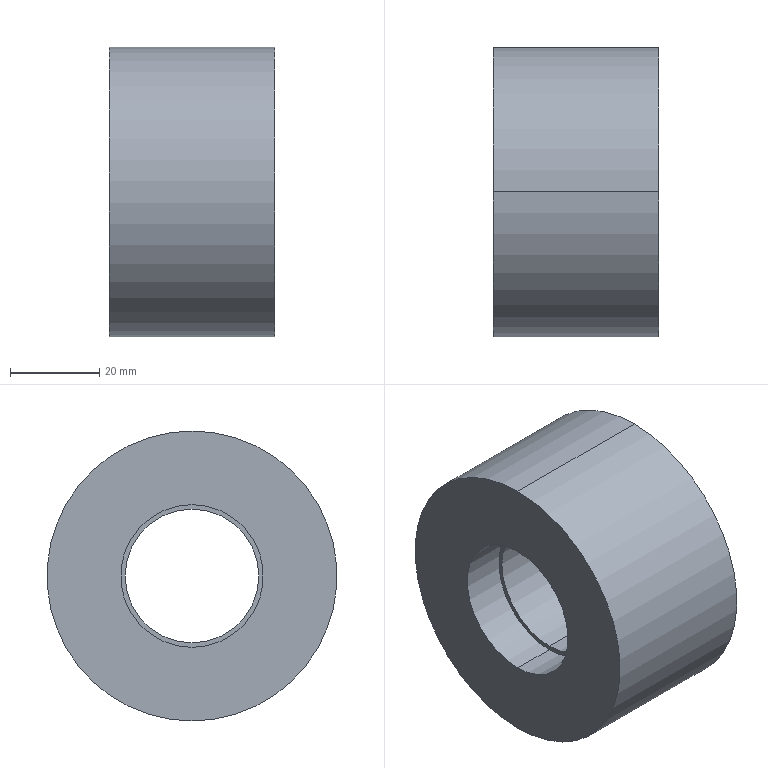Part | STEP file | 0245_Z_009_AFBD37-65_1 | 1 solid | 12 faces | box 37 x 65 x 65 mm | volume 94676 mm3 | cylinder 8 | plane 4 | commonest cylinder face diameters 32 x4 30 x2 65 x2
STEP:
#1=CARTESIAN_POINT('',(0.,0.,0.));
#2=DIRECTION('',(0.,0.,1.));
#3=DIRECTION('',(1.,0.,0.));
#4=AXIS2_PLACEMENT_3D('',#1,#2,#3);
#5=CARTESIAN_POINT('',(-18.5,0.,-32.5));
#6=VERTEX_POINT('',#5);
#7=CARTESIAN_POINT('',(-18.5,0.,32.5));
#8=VERTEX_POINT('',#7);
#9=CARTESIAN_POINT('',(-18.5,0.,0.));
#10=DIRECTION('',(1.,0.,0.));
#11=DIRECTION('',(0.,0.,-1.));
#12=AXIS2_PLACEMENT_3D('',#9,#10,#11);
#13=CIRCLE('',#12,32.5);
#14=CARTESIAN_POINT('',(0.,0.,0.));
#15=DIRECTION('',(1.,0.,0.));
#16=DIRECTION('',(0.,0.,-1.));
#17=AXIS2_PLACEMENT_3D('',#14,#15,#16);
#18=CYLINDRICAL_SURFACE('',#17,32.5);
#19=CARTESIAN_POINT('',(0.,-18.5));
#20=DIRECTION('',(1.,0.));
#21=VECTOR('',#20,1.);
#22=LINE('',#19,#21);
#23=(GEOMETRIC_REPRESENTATION_CONTEXT(2)PARAMETRIC_REPRESENTATION_CONTEXT()REPRESENTATION_CONTEXT('',''));
#24=DEFINITIONAL_REPRESENTATION('',(#22),#23);
#25=PCURVE('',#18,#24);
#26=CARTESIAN_POINT('',(-18.5,24.25,0.));
#27=DIRECTION('',(-1.,0.,0.));
#28=DIRECTION('',(0.,0.,1.));
#29=AXIS2_PLACEMENT_3D('',#26,#27,#28);
#30=PLANE('',#29);
#31=CARTESIAN_POINT('',(-32.5,-24.25));
#32=CARTESIAN_POINT('',(-32.5,32.042));
#33=CARTESIAN_POINT('',(16.25,3.896));
#34=CARTESIAN_POINT('',(65.,-24.25));
#35=CARTESIAN_POINT('',(16.25,-52.396));
#36=CARTESIAN_POINT('',(-32.5,-80.542));
#37=CARTESIAN_POINT('',(-32.5,-24.25));
#38=(BOUNDED_CURVE()B_SPLINE_CURVE(2,(#31,#32,#33,#34,#35,#36,#37),.UNSPECIFIED.,.T.,.F.)B_SPLINE_CURVE_WITH_KNOTS((1,2,2,2,2,1),(-2.094,0.,2.094,4.189,6.283,8.378),.UNSPECIFIED.)CURVE()GEOMETRIC_REPRESENTATION_ITEM()RATIONAL_B_SPLINE_CURVE((1.,0.5,1.,0.5,1.,0.5,1.))REPRESENTATION_ITEM(''));
#39=(GEOMETRIC_REPRESENTATION_CONTEXT(2)PARAMETRIC_REPRESENTATION_CONTEXT()REPRESENTATION_CONTEXT('',''));
#40=DEFINITIONAL_REPRESENTATION('',(#38),#39);
#41=PCURVE('',#30,#40);
#42=SURFACE_CURVE('',#13,(#25,#41),.PCURVE_S1.);
#43=EDGE_CURVE('',#6,#8,#42,.T.);
#44=ORIENTED_EDGE('',*,*,#43,.T.);
#45=CARTESIAN_POINT('',(18.5,0.,32.5));
#46=VERTEX_POINT('',#45);
#47=CARTESIAN_POINT('',(0.,0.,32.5));
#48=DIRECTION('',(1.,0.,0.));
#49=VECTOR('',#48,1.);
#50=LINE('',#47,#49);
#51=CARTESIAN_POINT('',(3.142,0.));
#52=DIRECTION('',(0.,1.));
#53=VECTOR('',#52,1.);
#54=LINE('',#51,#53);
#55=(GEOMETRIC_REPRESENTATION_CONTEXT(2)PARAMETRIC_REPRESENTATION_CONTEXT()REPRESENTATION_CONTEXT('',''));
#56=DEFINITIONAL_REPRESENTATION('',(#54),#55);
#57=PCURVE('',#18,#56);
#58=CARTESIAN_POINT('',(0.,0.,0.));
#59=DIRECTION('',(1.,0.,0.));
#60=DIRECTION('',(0.,0.,-1.));
#61=AXIS2_PLACEMENT_3D('',#58,#59,#60);
#62=CYLINDRICAL_SURFACE('',#61,32.5);
#63=CARTESIAN_POINT('',(3.142,0.));
#64=DIRECTION('',(0.,1.));
#65=VECTOR('',#64,1.);
#66=LINE('',#63,#65);
#67=(GEOMETRIC_REPRESENTATION_CONTEXT(2)PARAMETRIC_REPRESENTATION_CONTEXT()REPRESENTATION_CONTEXT('',''));
#68=DEFINITIONAL_REPRESENTATION('',(#66),#67);
#69=PCURVE('',#62,#68);
#70=SURFACE_CURVE('',#50,(#57,#69),.PCURVE_S1.);
#71=EDGE_CURVE('',#8,#46,#70,.T.);
#72=ORIENTED_EDGE('',*,*,#71,.T.);
#73=CARTESIAN_POINT('',(18.5,0.,-32.5));
#74=VERTEX_POINT('',#73);
#75=CARTESIAN_POINT('',(18.5,0.,0.));
#76=DIRECTION('',(-1.,0.,0.));
#77=DIRECTION('',(0.,0.,-1.));
#78=AXIS2_PLACEMENT_3D('',#75,#76,#77);
#79=CIRCLE('',#78,32.5);
#80=CARTESIAN_POINT('',(6.283,18.5));
#81=DIRECTION('',(-1.,0.));
#82=VECTOR('',#81,1.);
#83=LINE('',#80,#82);
#84=(GEOMETRIC_REPRESENTATION_CONTEXT(2)PARAMETRIC_REPRESENTATION_CONTEXT()REPRESENTATION_CONTEXT('',''));
#85=DEFINITIONAL_REPRESENTATION('',(#83),#84);
#86=PCURVE('',#18,#85);
#87=CARTESIAN_POINT('',(18.5,24.25,0.));
#88=DIRECTION('',(1.,0.,0.));
#89=DIRECTION('',(0.,0.,-1.));
#90=AXIS2_PLACEMENT_3D('',#87,#88,#89);
#91=PLANE('',#90);
#92=CARTESIAN_POINT('',(32.5,-24.25));
#93=CARTESIAN_POINT('',(32.5,-80.542));
#94=CARTESIAN_POINT('',(-16.25,-52.396));
#95=CARTESIAN_POINT('',(-65.,-24.25));
#96=CARTESIAN_POINT('',(-16.25,3.896));
#97=CARTESIAN_POINT('',(32.5,32.042));
#98=CARTESIAN_POINT('',(32.5,-24.25));
#99=(BOUNDED_CURVE()B_SPLINE_CURVE(2,(#92,#93,#94,#95,#96,#97,#98),.UNSPECIFIED.,.T.,.F.)B_SPLINE_CURVE_WITH_KNOTS((1,2,2,2,2,1),(-2.094,0.,2.094,4.189,6.283,8.378),.UNSPECIFIED.)CURVE()GEOMETRIC_REPRESENTATION_ITEM()RATIONAL_B_SPLINE_CURVE((1.,0.5,1.,0.5,1.,0.5,1.))REPRESENTATION_ITEM(''));
#100=(GEOMETRIC_REPRESENTATION_CONTEXT(2)PARAMETRIC_REPRESENTATION_CONTEXT()REPRESENTATION_CONTEXT('',''));
#101=DEFINITIONAL_REPRESENTATION('',(#99),#100);
#102=PCURVE('',#91,#101);
#103=SURFACE_CURVE('',#79,(#86,#102),.PCURVE_S1.);
#104=EDGE_CURVE('',#46,#74,#103,.T.);
#105=ORIENTED_EDGE('',*,*,#104,.T.);
#106=CARTESIAN_POINT('',(0.,0.,-32.5));
#107=DIRECTION('',(1.,0.,0.));
#108=VECTOR('',#107,1.);
#109=LINE('',#106,#108);
#110=CARTESIAN_POINT('',(0.,0.));
#111=DIRECTION('',(0.,1.));
#112=VECTOR('',#111,1.);
#113=LINE('',#110,#112);
#114=(GEOMETRIC_REPRESENTATION_CONTEXT(2)PARAMETRIC_REPRESENTATION_CONTEXT()REPRESENTATION_CONTEXT('',''));
#115=DEFINITIONAL_REPRESENTATION('',(#113),#114);
#116=PCURVE('',#18,#115);
#117=CARTESIAN_POINT('',(6.283,0.));
#118=DIRECTION('',(0.,1.));
#119=VECTOR('',#118,1.);
#120=LINE('',#117,#119);
#121=(GEOMETRIC_REPRESENTATION_CONTEXT(2)PARAMETRIC_REPRESENTATION_CONTEXT()REPRESENTATION_CONTEXT('',''));
#122=DEFINITIONAL_REPRESENTATION('',(#120),#121);
#123=PCURVE('',#62,#122);
#124=SURFACE_CURVE('',#109,(#116,#123),.PCURVE_S1.);
#125=EDGE_CURVE('',#6,#74,#124,.T.);
#126=ORIENTED_EDGE('',*,*,#125,.F.);
#127=EDGE_LOOP('',(#44,#72,#105,#126));
#128=FACE_BOUND('',#127,.T.);
#129=ADVANCED_FACE('',(#128),#18,.T.);
#130=CARTESIAN_POINT('',(-18.5,0.,-16.));
#131=VERTEX_POINT('',#130);
#132=CARTESIAN_POINT('',(-8.5,0.,-16.));
#133=VERTEX_POINT('',#132);
#134=CARTESIAN_POINT('',(-13.5,0.,-16.));
#135=DIRECTION('',(1.,0.,0.));
#136=VECTOR('',#135,1.);
#137=LINE('',#134,#136);
#138=CARTESIAN_POINT('',(-13.5,0.,0.));
#139=DIRECTION('',(1.,0.,0.));
#140=DIRECTION('',(0.,0.,-1.));
#141=AXIS2_PLACEMENT_3D('',#138,#139,#140);
#142=CYLINDRICAL_SURFACE('',#141,16.);
#143=CARTESIAN_POINT('',(6.283,0.));
#144=DIRECTION('',(0.,1.));
#145=VECTOR('',#144,1.);
#146=LINE('',#143,#145);
#147=(GEOMETRIC_REPRESENTATION_CONTEXT(2)PARAMETRIC_REPRESENTATION_CONTEXT()REPRESENTATION_CONTEXT('',''));
#148=DEFINITIONAL_REPRESENTATION('',(#146),#147);
#149=PCURVE('',#142,#148);
#150=CARTESIAN_POINT('',(-13.5,0.,0.));
#151=DIRECTION('',(1.,0.,0.));
#152=DIRECTION('',(0.,0.,-1.));
#153=AXIS2_PLACEMENT_3D('',#150,#151,#152);
#154=CYLINDRICAL_SURFACE('',#153,16.);
#155=CARTESIAN_POINT('',(0.,0.));
#156=DIRECTION('',(0.,1.));
#157=VECTOR('',#156,1.);
#158=LINE('',#155,#157);
#159=(GEOMETRIC_REPRESENTATION_CONTEXT(2)PARAMETRIC_REPRESENTATION_CONTEXT()REPRESENTATION_CONTEXT('',''));
#160=DEFINITIONAL_REPRESENTATION('',(#158),#159);
#161=PCURVE('',#154,#160);
#162=SURFACE_CURVE('',#137,(#149,#161),.PCURVE_S1.);
#163=EDGE_CURVE('',#131,#133,#162,.T.);
#164=ORIENTED_EDGE('',*,*,#163,.T.);
#165=CARTESIAN_POINT('',(-8.5,0.,16.));
#166=VERTEX_POINT('',#165);
#167=CARTESIAN_POINT('',(-8.5,0.,0.));
#168=DIRECTION('',(-1.,0.,0.));
#169=DIRECTION('',(0.,0.,-1.));
#170=AXIS2_PLACEMENT_3D('',#167,#168,#169);
#171=CIRCLE('',#170,16.);
#172=CARTESIAN_POINT('',(6.283,5.));
#173=DIRECTION('',(-1.,0.));
#174=VECTOR('',#173,1.);
#175=LINE('',#172,#174);
#176=(GEOMETRIC_REPRESENTATION_CONTEXT(2)PARAMETRIC_REPRESENTATION_CONTEXT()REPRESENTATION_CONTEXT('',''));
#177=DEFINITIONAL_REPRESENTATION('',(#175),#176);
#178=PCURVE('',#142,#177);
#179=CARTESIAN_POINT('',(-8.5,15.5,0.));
#180=DIRECTION('',(-1.,0.,0.));
#181=DIRECTION('',(0.,0.,1.));
#182=AXIS2_PLACEMENT_3D('',#179,#180,#181);
#183=PLANE('',#182);
#184=CARTESIAN_POINT('',(0.,-15.5));
#185=DIRECTION('',(-1.,0.));
#186=AXIS2_PLACEMENT_2D('',#184,#185);
#187=CIRCLE('',#186,16.);
#188=(GEOMETRIC_REPRESENTATION_CONTEXT(2)PARAMETRIC_REPRESENTATION_CONTEXT()REPRESENTATION_CONTEXT('',''));
#189=DEFINITIONAL_REPRESENTATION('',(#187),#188);
#190=PCURVE('',#183,#189);
#191=SURFACE_CURVE('',#171,(#178,#190),.PCURVE_S1.);
#192=EDGE_CURVE('',#133,#166,#191,.T.);
#193=ORIENTED_EDGE('',*,*,#192,.T.);
#194=CARTESIAN_POINT('',(-18.5,0.,16.));
#195=VERTEX_POINT('',#194);
#196=CARTESIAN_POINT('',(-13.5,0.,16.));
#197=DIRECTION('',(1.,0.,0.));
#198=VECTOR('',#197,1.);
#199=LINE('',#196,#198);
#200=CARTESIAN_POINT('',(3.142,0.));
#201=DIRECTION('',(0.,1.));
#202=VECTOR('',#201,1.);
#203=LINE('',#200,#202);
#204=(GEOMETRIC_REPRESENTATION_CONTEXT(2)PARAMETRIC_REPRESENTATION_CONTEXT()REPRESENTATION_CONTEXT('',''));
#205=DEFINITIONAL_REPRESENTATION('',(#203),#204);
#206=PCURVE('',#142,#205);
#207=CARTESIAN_POINT('',(3.142,0.));
#208=DIRECTION('',(0.,1.));
#209=VECTOR('',#208,1.);
#210=LINE('',#207,#209);
#211=(GEOMETRIC_REPRESENTATION_CONTEXT(2)PARAMETRIC_REPRESENTATION_CONTEXT()REPRESENTATION_CONTEXT('',''));
#212=DEFINITIONAL_REPRESENTATION('',(#210),#211);
#213=PCURVE('',#154,#212);
#214=SURFACE_CURVE('',#199,(#206,#213),.PCURVE_S1.);
#215=EDGE_CURVE('',#195,#166,#214,.T.);
#216=ORIENTED_EDGE('',*,*,#215,.F.);
#217=CARTESIAN_POINT('',(-18.5,0.,0.));
#218=DIRECTION('',(1.,0.,0.));
#219=DIRECTION('',(0.,0.,-1.));
#220=AXIS2_PLACEMENT_3D('',#217,#218,#219);
#221=CIRCLE('',#220,16.);
#222=CARTESIAN_POINT('',(0.,-5.));
#223=DIRECTION('',(1.,0.));
#224=VECTOR('',#223,1.);
#225=LINE('',#222,#224);
#226=(GEOMETRIC_REPRESENTATION_CONTEXT(2)PARAMETRIC_REPRESENTATION_CONTEXT()REPRESENTATION_CONTEXT('',''));
#227=DEFINITIONAL_REPRESENTATION('',(#225),#226);
#228=PCURVE('',#142,#227);
#229=CARTESIAN_POINT('',(-16.,-24.25));
#230=CARTESIAN_POINT('',(-16.,3.463));
#231=CARTESIAN_POINT('',(8.,-10.394));
#232=CARTESIAN_POINT('',(32.,-24.25));
#233=CARTESIAN_POINT('',(8.,-38.106));
#234=CARTESIAN_POINT('',(-16.,-51.963));
#235=CARTESIAN_POINT('',(-16.,-24.25));
#236=(BOUNDED_CURVE()B_SPLINE_CURVE(2,(#229,#230,#231,#232,#233,#234,#235),.UNSPECIFIED.,.T.,.F.)B_SPLINE_CURVE_WITH_KNOTS((1,2,2,2,2,1),(-2.094,0.,2.094,4.189,6.283,8.378),.UNSPECIFIED.)CURVE()GEOMETRIC_REPRESENTATION_ITEM()RATIONAL_B_SPLINE_CURVE((1.,0.5,1.,0.5,1.,0.5,1.))REPRESENTATION_ITEM(''));
#237=(GEOMETRIC_REPRESENTATION_CONTEXT(2)PARAMETRIC_REPRESENTATION_CONTEXT()REPRESENTATION_CONTEXT('',''));
#238=DEFINITIONAL_REPRESENTATION('',(#236),#237);
#239=PCURVE('',#30,#238);
#240=SURFACE_CURVE('',#221,(#228,#239),.PCURVE_S1.);
#241=EDGE_CURVE('',#195,#131,#240,.T.);
#242=ORIENTED_EDGE('',*,*,#241,.T.);
#243=EDGE_LOOP('',(#164,#193,#216,#242));
#244=FACE_BOUND('',#243,.F.);
#245=ADVANCED_FACE('',(#244),#142,.F.);
#246=CARTESIAN_POINT('',(8.5,0.,-16.));
#247=VERTEX_POINT('',#246);
#248=CARTESIAN_POINT('',(18.5,0.,-16.));
#249=VERTEX_POINT('',#248);
#250=CARTESIAN_POINT('',(13.5,0.,-16.));
#251=DIRECTION('',(1.,0.,0.));
#252=VECTOR('',#251,1.);
#253=LINE('',#250,#252);
#254=CARTESIAN_POINT('',(13.5,0.,0.));
#255=DIRECTION('',(1.,0.,0.));
#256=DIRECTION('',(0.,0.,-1.));
#257=AXIS2_PLACEMENT_3D('',#254,#255,#256);
#258=CYLINDRICAL_SURFACE('',#257,16.);
#259=CARTESIAN_POINT('',(6.283,0.));
#260=DIRECTION('',(0.,1.));
#261=VECTOR('',#260,1.);
#262=LINE('',#259,#261);
#263=(GEOMETRIC_REPRESENTATION_CONTEXT(2)PARAMETRIC_REPRESENTATION_CONTEXT()REPRESENTATION_CONTEXT('',''));
#264=DEFINITIONAL_REPRESENTATION('',(#262),#263);
#265=PCURVE('',#258,#264);
#266=CARTESIAN_POINT('',(13.5,0.,0.));
#267=DIRECTION('',(1.,0.,0.));
#268=DIRECTION('',(0.,0.,-1.));
#269=AXIS2_PLACEMENT_3D('',#266,#267,#268);
#270=CYLINDRICAL_SURFACE('',#269,16.);
#271=CARTESIAN_POINT('',(0.,0.));
#272=DIRECTION('',(0.,1.));
#273=VECTOR('',#272,1.);
#274=LINE('',#271,#273);
#275=(GEOMETRIC_REPRESENTATION_CONTEXT(2)PARAMETRIC_REPRESENTATION_CONTEXT()REPRESENTATION_CONTEXT('',''));
#276=DEFINITIONAL_REPRESENTATION('',(#274),#275);
#277=PCURVE('',#270,#276);
#278=SURFACE_CURVE('',#253,(#265,#277),.PCURVE_S1.);
#279=EDGE_CURVE('',#247,#249,#278,.T.);
#280=ORIENTED_EDGE('',*,*,#279,.T.);
#281=CARTESIAN_POINT('',(18.5,0.,16.));
#282=VERTEX_POINT('',#281);
#283=CARTESIAN_POINT('',(18.5,0.,0.));
#284=DIRECTION('',(-1.,0.,0.));
#285=DIRECTION('',(0.,0.,-1.));
#286=AXIS2_PLACEMENT_3D('',#283,#284,#285);
#287=CIRCLE('',#286,16.);
#288=CARTESIAN_POINT('',(6.283,5.));
#289=DIRECTION('',(-1.,0.));
#290=VECTOR('',#289,1.);
#291=LINE('',#288,#290);
#292=(GEOMETRIC_REPRESENTATION_CONTEXT(2)PARAMETRIC_REPRESENTATION_CONTEXT()REPRESENTATION_CONTEXT('',''));
#293=DEFINITIONAL_REPRESENTATION('',(#291),#292);
#294=PCURVE('',#258,#293);
#295=CARTESIAN_POINT('',(16.,-24.25));
#296=CARTESIAN_POINT('',(16.,-51.963));
#297=CARTESIAN_POINT('',(-8.,-38.106));
#298=CARTESIAN_POINT('',(-32.,-24.25));
#299=CARTESIAN_POINT('',(-8.,-10.394));
#300=CARTESIAN_POINT('',(16.,3.463));
#301=CARTESIAN_POINT('',(16.,-24.25));
#302=(BOUNDED_CURVE()B_SPLINE_CURVE(2,(#295,#296,#297,#298,#299,#300,#301),.UNSPECIFIED.,.T.,.F.)B_SPLINE_CURVE_WITH_KNOTS((1,2,2,2,2,1),(-2.094,0.,2.094,4.189,6.283,8.378),.UNSPECIFIED.)CURVE()GEOMETRIC_REPRESENTATION_ITEM()RATIONAL_B_SPLINE_CURVE((1.,0.5,1.,0.5,1.,0.5,1.))REPRESENTATION_ITEM(''));
#303=(GEOMETRIC_REPRESENTATION_CONTEXT(2)PARAMETRIC_REPRESENTATION_CONTEXT()REPRESENTATION_CONTEXT('',''));
#304=DEFINITIONAL_REPRESENTATION('',(#302),#303);
#305=PCURVE('',#91,#304);
#306=SURFACE_CURVE('',#287,(#294,#305),.PCURVE_S1.);
#307=EDGE_CURVE('',#249,#282,#306,.T.);
#308=ORIENTED_EDGE('',*,*,#307,.T.);
#309=CARTESIAN_POINT('',(8.5,0.,16.));
#310=VERTEX_POINT('',#309);
#311=CARTESIAN_POINT('',(13.5,0.,16.));
#312=DIRECTION('',(1.,0.,0.));
#313=VECTOR('',#312,1.);
#314=LINE('',#311,#313);
#315=CARTESIAN_POINT('',(3.142,0.));
#316=DIRECTION('',(0.,1.));
#317=VECTOR('',#316,1.);
#318=LINE('',#315,#317);
#319=(GEOMETRIC_REPRESENTATION_CONTEXT(2)PARAMETRIC_REPRESENTATION_CONTEXT()REPRESENTATION_CONTEXT('',''));
#320=DEFINITIONAL_REPRESENTATION('',(#318),#319);
#321=PCURVE('',#258,#320);
#322=CARTESIAN_POINT('',(3.142,0.));
#323=DIRECTION('',(0.,1.));
#324=VECTOR('',#323,1.);
#325=LINE('',#322,#324);
#326=(GEOMETRIC_REPRESENTATION_CONTEXT(2)PARAMETRIC_REPRESENTATION_CONTEXT()REPRESENTATION_CONTEXT('',''));
#327=DEFINITIONAL_REPRESENTATION('',(#325),#326);
#328=PCURVE('',#270,#327);
#329=SURFACE_CURVE('',#314,(#321,#328),.PCURVE_S1.);
#330=EDGE_CURVE('',#310,#282,#329,.T.);
#331=ORIENTED_EDGE('',*,*,#330,.F.);
#332=CARTESIAN_POINT('',(8.5,0.,0.));
#333=DIRECTION('',(1.,0.,0.));
#334=DIRECTION('',(0.,0.,-1.));
#335=AXIS2_PLACEMENT_3D('',#332,#333,#334);
#336=CIRCLE('',#335,16.);
#337=CARTESIAN_POINT('',(0.,-5.));
#338=DIRECTION('',(1.,0.));
#339=VECTOR('',#338,1.);
#340=LINE('',#337,#339);
#341=(GEOMETRIC_REPRESENTATION_CONTEXT(2)PARAMETRIC_REPRESENTATION_CONTEXT()REPRESENTATION_CONTEXT('',''));
#342=DEFINITIONAL_REPRESENTATION('',(#340),#341);
#343=PCURVE('',#258,#342);
#344=CARTESIAN_POINT('',(8.5,15.5,0.));
#345=DIRECTION('',(1.,0.,0.));
#346=DIRECTION('',(0.,0.,-1.));
#347=AXIS2_PLACEMENT_3D('',#344,#345,#346);
#348=PLANE('',#347);
#349=CARTESIAN_POINT('',(0.,-15.5));
#350=DIRECTION('',(1.,0.));
#351=AXIS2_PLACEMENT_2D('',#349,#350);
#352=CIRCLE('',#351,16.);
#353=(GEOMETRIC_REPRESENTATION_CONTEXT(2)PARAMETRIC_REPRESENTATION_CONTEXT()REPRESENTATION_CONTEXT('',''));
#354=DEFINITIONAL_REPRESENTATION('',(#352),#353);
#355=PCURVE('',#348,#354);
#356=SURFACE_CURVE('',#336,(#343,#355),.PCURVE_S1.);
#357=EDGE_CURVE('',#310,#247,#356,.T.);
#358=ORIENTED_EDGE('',*,*,#357,.T.);
#359=EDGE_LOOP('',(#280,#308,#331,#358));
#360=FACE_BOUND('',#359,.F.);
#361=ADVANCED_FACE('',(#360),#258,.F.);
#362=CARTESIAN_POINT('',(-8.5,0.,-15.));
#363=VERTEX_POINT('',#362);
#364=CARTESIAN_POINT('',(8.5,0.,-15.));
#365=VERTEX_POINT('',#364);
#366=CARTESIAN_POINT('',(0.,0.,-15.));
#367=DIRECTION('',(1.,0.,0.));
#368=VECTOR('',#367,1.);
#369=LINE('',#366,#368);
#370=CARTESIAN_POINT('',(0.,0.,0.));
#371=DIRECTION('',(1.,0.,0.));
#372=DIRECTION('',(0.,0.,-1.));
#373=AXIS2_PLACEMENT_3D('',#370,#371,#372);
#374=CYLINDRICAL_SURFACE('',#373,15.);
#375=CARTESIAN_POINT('',(6.283,0.));
#376=DIRECTION('',(0.,1.));
#377=VECTOR('',#376,1.);
#378=LINE('',#375,#377);
#379=(GEOMETRIC_REPRESENTATION_CONTEXT(2)PARAMETRIC_REPRESENTATION_CONTEXT()REPRESENTATION_CONTEXT('',''));
#380=DEFINITIONAL_REPRESENTATION('',(#378),#379);
#381=PCURVE('',#374,#380);
#382=CARTESIAN_POINT('',(0.,0.,0.));
#383=DIRECTION('',(1.,0.,0.));
#384=DIRECTION('',(0.,0.,-1.));
#385=AXIS2_PLACEMENT_3D('',#382,#383,#384);
#386=CYLINDRICAL_SURFACE('',#385,15.);
#387=CARTESIAN_POINT('',(0.,0.));
#388=DIRECTION('',(0.,1.));
#389=VECTOR('',#388,1.);
#390=LINE('',#387,#389);
#391=(GEOMETRIC_REPRESENTATION_CONTEXT(2)PARAMETRIC_REPRESENTATION_CONTEXT()REPRESENTATION_CONTEXT('',''));
#392=DEFINITIONAL_REPRESENTATION('',(#390),#391);
#393=PCURVE('',#386,#392);
#394=SURFACE_CURVE('',#369,(#381,#393),.PCURVE_S1.);
#395=EDGE_CURVE('',#363,#365,#394,.T.);
#396=ORIENTED_EDGE('',*,*,#395,.T.);
#397=CARTESIAN_POINT('',(8.5,0.,15.));
#398=VERTEX_POINT('',#397);
#399=CARTESIAN_POINT('',(8.5,0.,0.));
#400=DIRECTION('',(-1.,0.,0.));
#401=DIRECTION('',(0.,0.,-1.));
#402=AXIS2_PLACEMENT_3D('',#399,#400,#401);
#403=CIRCLE('',#402,15.);
#404=CARTESIAN_POINT('',(6.283,8.5));
#405=DIRECTION('',(-1.,0.));
#406=VECTOR('',#405,1.);
#407=LINE('',#404,#406);
#408=(GEOMETRIC_REPRESENTATION_CONTEXT(2)PARAMETRIC_REPRESENTATION_CONTEXT()REPRESENTATION_CONTEXT('',''));
#409=DEFINITIONAL_REPRESENTATION('',(#407),#408);
#410=PCURVE('',#374,#409);
#411=CARTESIAN_POINT('',(15.,-15.5));
#412=CARTESIAN_POINT('',(15.,-41.481));
#413=CARTESIAN_POINT('',(-7.5,-28.49));
#414=CARTESIAN_POINT('',(-30.,-15.5));
#415=CARTESIAN_POINT('',(-7.5,-2.51));
#416=CARTESIAN_POINT('',(15.,10.481));
#417=CARTESIAN_POINT('',(15.,-15.5));
#418=(BOUNDED_CURVE()B_SPLINE_CURVE(2,(#411,#412,#413,#414,#415,#416,#417),.UNSPECIFIED.,.T.,.F.)B_SPLINE_CURVE_WITH_KNOTS((1,2,2,2,2,1),(-2.094,0.,2.094,4.189,6.283,8.378),.UNSPECIFIED.)CURVE()GEOMETRIC_REPRESENTATION_ITEM()RATIONAL_B_SPLINE_CURVE((1.,0.5,1.,0.5,1.,0.5,1.))REPRESENTATION_ITEM(''));
#419=(GEOMETRIC_REPRESENTATION_CONTEXT(2)PARAMETRIC_REPRESENTATION_CONTEXT()REPRESENTATION_CONTEXT('',''));
#420=DEFINITIONAL_REPRESENTATION('',(#418),#419);
#421=PCURVE('',#348,#420);
#422=SURFACE_CURVE('',#403,(#410,#421),.PCURVE_S1.);
#423=EDGE_CURVE('',#365,#398,#422,.T.);
#424=ORIENTED_EDGE('',*,*,#423,.T.);
#425=CARTESIAN_POINT('',(-8.5,0.,15.));
#426=VERTEX_POINT('',#425);
#427=CARTESIAN_POINT('',(0.,0.,15.));
#428=DIRECTION('',(1.,0.,0.));
#429=VECTOR('',#428,1.);
#430=LINE('',#427,#429);
#431=CARTESIAN_POINT('',(3.142,0.));
#432=DIRECTION('',(0.,1.));
#433=VECTOR('',#432,1.);
#434=LINE('',#431,#433);
#435=(GEOMETRIC_REPRESENTATION_CONTEXT(2)PARAMETRIC_REPRESENTATION_CONTEXT()REPRESENTATION_CONTEXT('',''));
#436=DEFINITIONAL_REPRESENTATION('',(#434),#435);
#437=PCURVE('',#374,#436);
#438=CARTESIAN_POINT('',(3.142,0.));
#439=DIRECTION('',(0.,1.));
#440=VECTOR('',#439,1.);
#441=LINE('',#438,#440);
#442=(GEOMETRIC_REPRESENTATION_CONTEXT(2)PARAMETRIC_REPRESENTATION_CONTEXT()REPRESENTATION_CONTEXT('',''));
#443=DEFINITIONAL_REPRESENTATION('',(#441),#442);
#444=PCURVE('',#386,#443);
#445=SURFACE_CURVE('',#430,(#437,#444),.PCURVE_S1.);
#446=EDGE_CURVE('',#426,#398,#445,.T.);
#447=ORIENTED_EDGE('',*,*,#446,.F.);
#448=CARTESIAN_POINT('',(-8.5,0.,0.));
#449=DIRECTION('',(1.,0.,0.));
#450=DIRECTION('',(0.,0.,-1.));
#451=AXIS2_PLACEMENT_3D('',#448,#449,#450);
#452=CIRCLE('',#451,15.);
#453=CARTESIAN_POINT('',(0.,-8.5));
#454=DIRECTION('',(1.,0.));
#455=VECTOR('',#454,1.);
#456=LINE('',#453,#455);
#457=(GEOMETRIC_REPRESENTATION_CONTEXT(2)PARAMETRIC_REPRESENTATION_CONTEXT()REPRESENTATION_CONTEXT('',''));
#458=DEFINITIONAL_REPRESENTATION('',(#456),#457);
#459=PCURVE('',#374,#458);
#460=CARTESIAN_POINT('',(-15.,-15.5));
#461=CARTESIAN_POINT('',(-15.,10.481));
#462=CARTESIAN_POINT('',(7.5,-2.51));
#463=CARTESIAN_POINT('',(30.,-15.5));
#464=CARTESIAN_POINT('',(7.5,-28.49));
#465=CARTESIAN_POINT('',(-15.,-41.481));
#466=CARTESIAN_POINT('',(-15.,-15.5));
#467=(BOUNDED_CURVE()B_SPLINE_CURVE(2,(#460,#461,#462,#463,#464,#465,#466),.UNSPECIFIED.,.T.,.F.)B_SPLINE_CURVE_WITH_KNOTS((1,2,2,2,2,1),(-2.094,0.,2.094,4.189,6.283,8.378),.UNSPECIFIED.)CURVE()GEOMETRIC_REPRESENTATION_ITEM()RATIONAL_B_SPLINE_CURVE((1.,0.5,1.,0.5,1.,0.5,1.))REPRESENTATION_ITEM(''));
#468=(GEOMETRIC_REPRESENTATION_CONTEXT(2)PARAMETRIC_REPRESENTATION_CONTEXT()REPRESENTATION_CONTEXT('',''));
#469=DEFINITIONAL_REPRESENTATION('',(#467),#468);
#470=PCURVE('',#183,#469);
#471=SURFACE_CURVE('',#452,(#459,#470),.PCURVE_S1.);
#472=EDGE_CURVE('',#426,#363,#471,.T.);
#473=ORIENTED_EDGE('',*,*,#472,.T.);
#474=EDGE_LOOP('',(#396,#424,#447,#473));
#475=FACE_BOUND('',#474,.F.);
#476=ADVANCED_FACE('',(#475),#374,.F.);
#477=ORIENTED_EDGE('',*,*,#71,.F.);
#478=CARTESIAN_POINT('',(-18.5,0.,0.));
#479=DIRECTION('',(1.,0.,0.));
#480=DIRECTION('',(0.,0.,-1.));
#481=AXIS2_PLACEMENT_3D('',#478,#479,#480);
#482=CIRCLE('',#481,32.5);
#483=CARTESIAN_POINT('',(0.,-18.5));
#484=DIRECTION('',(1.,0.));
#485=VECTOR('',#484,1.);
#486=LINE('',#483,#485);
#487=(GEOMETRIC_REPRESENTATION_CONTEXT(2)PARAMETRIC_REPRESENTATION_CONTEXT()REPRESENTATION_CONTEXT('',''));
#488=DEFINITIONAL_REPRESENTATION('',(#486),#487);
#489=PCURVE('',#62,#488);
#490=CARTESIAN_POINT('',(-32.5,-24.25));
#491=CARTESIAN_POINT('',(-32.5,32.042));
#492=CARTESIAN_POINT('',(16.25,3.896));
#493=CARTESIAN_POINT('',(65.,-24.25));
#494=CARTESIAN_POINT('',(16.25,-52.396));
#495=CARTESIAN_POINT('',(-32.5,-80.542));
#496=CARTESIAN_POINT('',(-32.5,-24.25));
#497=(BOUNDED_CURVE()B_SPLINE_CURVE(2,(#490,#491,#492,#493,#494,#495,#496),.UNSPECIFIED.,.T.,.F.)B_SPLINE_CURVE_WITH_KNOTS((1,2,2,2,2,1),(-2.094,0.,2.094,4.189,6.283,8.378),.UNSPECIFIED.)CURVE()GEOMETRIC_REPRESENTATION_ITEM()RATIONAL_B_SPLINE_CURVE((1.,0.5,1.,0.5,1.,0.5,1.))REPRESENTATION_ITEM(''));
#498=(GEOMETRIC_REPRESENTATION_CONTEXT(2)PARAMETRIC_REPRESENTATION_CONTEXT()REPRESENTATION_CONTEXT('',''));
#499=DEFINITIONAL_REPRESENTATION('',(#497),#498);
#500=PCURVE('',#30,#499);
#501=SURFACE_CURVE('',#482,(#489,#500),.PCURVE_S1.);
#502=EDGE_CURVE('',#8,#6,#501,.T.);
#503=ORIENTED_EDGE('',*,*,#502,.T.);
#504=ORIENTED_EDGE('',*,*,#125,.T.);
#505=CARTESIAN_POINT('',(18.5,0.,0.));
#506=DIRECTION('',(-1.,0.,0.));
#507=DIRECTION('',(0.,0.,-1.));
#508=AXIS2_PLACEMENT_3D('',#505,#506,#507);
#509=CIRCLE('',#508,32.5);
#510=CARTESIAN_POINT('',(6.283,18.5));
#511=DIRECTION('',(-1.,0.));
#512=VECTOR('',#511,1.);
#513=LINE('',#510,#512);
#514=(GEOMETRIC_REPRESENTATION_CONTEXT(2)PARAMETRIC_REPRESENTATION_CONTEXT()REPRESENTATION_CONTEXT('',''));
#515=DEFINITIONAL_REPRESENTATION('',(#513),#514);
#516=PCURVE('',#62,#515);
#517=CARTESIAN_POINT('',(32.5,-24.25));
#518=CARTESIAN_POINT('',(32.5,-80.542));
#519=CARTESIAN_POINT('',(-16.25,-52.396));
#520=CARTESIAN_POINT('',(-65.,-24.25));
#521=CARTESIAN_POINT('',(-16.25,3.896));
#522=CARTESIAN_POINT('',(32.5,32.042));
#523=CARTESIAN_POINT('',(32.5,-24.25));
#524=(BOUNDED_CURVE()B_SPLINE_CURVE(2,(#517,#518,#519,#520,#521,#522,#523),.UNSPECIFIED.,.T.,.F.)B_SPLINE_CURVE_WITH_KNOTS((1,2,2,2,2,1),(-2.094,0.,2.094,4.189,6.283,8.378),.UNSPECIFIED.)CURVE()GEOMETRIC_REPRESENTATION_ITEM()RATIONAL_B_SPLINE_CURVE((1.,0.5,1.,0.5,1.,0.5,1.))REPRESENTATION_ITEM(''));
#525=(GEOMETRIC_REPRESENTATION_CONTEXT(2)PARAMETRIC_REPRESENTATION_CONTEXT()REPRESENTATION_CONTEXT('',''));
#526=DEFINITIONAL_REPRESENTATION('',(#524),#525);
#527=PCURVE('',#91,#526);
#528=SURFACE_CURVE('',#509,(#516,#527),.PCURVE_S1.);
#529=EDGE_CURVE('',#74,#46,#528,.T.);
#530=ORIENTED_EDGE('',*,*,#529,.T.);
#531=EDGE_LOOP('',(#477,#503,#504,#530));
#532=FACE_BOUND('',#531,.T.);
#533=ADVANCED_FACE('',(#532),#62,.T.);
#534=ORIENTED_EDGE('',*,*,#43,.F.);
#535=ORIENTED_EDGE('',*,*,#502,.F.);
#536=EDGE_LOOP('',(#534,#535));
#537=FACE_BOUND('',#536,.T.);
#538=CARTESIAN_POINT('',(-18.5,0.,0.));
#539=DIRECTION('',(1.,0.,0.));
#540=DIRECTION('',(0.,0.,-1.));
#541=AXIS2_PLACEMENT_3D('',#538,#539,#540);
#542=CIRCLE('',#541,16.);
#543=CARTESIAN_POINT('',(-16.,-24.25));
#544=CARTESIAN_POINT('',(-16.,3.463));
#545=CARTESIAN_POINT('',(8.,-10.394));
#546=CARTESIAN_POINT('',(32.,-24.25));
#547=CARTESIAN_POINT('',(8.,-38.106));
#548=CARTESIAN_POINT('',(-16.,-51.963));
#549=CARTESIAN_POINT('',(-16.,-24.25));
#550=(BOUNDED_CURVE()B_SPLINE_CURVE(2,(#543,#544,#545,#546,#547,#548,#549),.UNSPECIFIED.,.T.,.F.)B_SPLINE_CURVE_WITH_KNOTS((1,2,2,2,2,1),(-2.094,0.,2.094,4.189,6.283,8.378),.UNSPECIFIED.)CURVE()GEOMETRIC_REPRESENTATION_ITEM()RATIONAL_B_SPLINE_CURVE((1.,0.5,1.,0.5,1.,0.5,1.))REPRESENTATION_ITEM(''));
#551=(GEOMETRIC_REPRESENTATION_CONTEXT(2)PARAMETRIC_REPRESENTATION_CONTEXT()REPRESENTATION_CONTEXT('',''));
#552=DEFINITIONAL_REPRESENTATION('',(#550),#551);
#553=PCURVE('',#30,#552);
#554=CARTESIAN_POINT('',(0.,-5.));
#555=DIRECTION('',(1.,0.));
#556=VECTOR('',#555,1.);
#557=LINE('',#554,#556);
#558=(GEOMETRIC_REPRESENTATION_CONTEXT(2)PARAMETRIC_REPRESENTATION_CONTEXT()REPRESENTATION_CONTEXT('',''));
#559=DEFINITIONAL_REPRESENTATION('',(#557),#558);
#560=PCURVE('',#154,#559);
#561=SURFACE_CURVE('',#542,(#553,#560),.PCURVE_S1.);
#562=EDGE_CURVE('',#131,#195,#561,.T.);
#563=ORIENTED_EDGE('',*,*,#562,.T.);
#564=ORIENTED_EDGE('',*,*,#241,.T.);
#565=EDGE_LOOP('',(#563,#564));
#566=FACE_BOUND('',#565,.T.);
#567=ADVANCED_FACE('',(#537,#566),#30,.T.);
#568=ORIENTED_EDGE('',*,*,#307,.T.);
#569=CARTESIAN_POINT('',(18.5,0.,0.));
#570=DIRECTION('',(-1.,0.,0.));
#571=DIRECTION('',(0.,0.,-1.));
#572=AXIS2_PLACEMENT_3D('',#569,#570,#571);
#573=CIRCLE('',#572,16.);
#574=CARTESIAN_POINT('',(16.,-24.25));
#575=CARTESIAN_POINT('',(16.,-51.963));
#576=CARTESIAN_POINT('',(-8.,-38.106));
#577=CARTESIAN_POINT('',(-32.,-24.25));
#578=CARTESIAN_POINT('',(-8.,-10.394));
#579=CARTESIAN_POINT('',(16.,3.463));
#580=CARTESIAN_POINT('',(16.,-24.25));
#581=(BOUNDED_CURVE()B_SPLINE_CURVE(2,(#574,#575,#576,#577,#578,#579,#580),.UNSPECIFIED.,.T.,.F.)B_SPLINE_CURVE_WITH_KNOTS((1,2,2,2,2,1),(-2.094,0.,2.094,4.189,6.283,8.378),.UNSPECIFIED.)CURVE()GEOMETRIC_REPRESENTATION_ITEM()RATIONAL_B_SPLINE_CURVE((1.,0.5,1.,0.5,1.,0.5,1.))REPRESENTATION_ITEM(''));
#582=(GEOMETRIC_REPRESENTATION_CONTEXT(2)PARAMETRIC_REPRESENTATION_CONTEXT()REPRESENTATION_CONTEXT('',''));
#583=DEFINITIONAL_REPRESENTATION('',(#581),#582);
#584=PCURVE('',#91,#583);
#585=CARTESIAN_POINT('',(6.283,5.));
#586=DIRECTION('',(-1.,0.));
#587=VECTOR('',#586,1.);
#588=LINE('',#585,#587);
#589=(GEOMETRIC_REPRESENTATION_CONTEXT(2)PARAMETRIC_REPRESENTATION_CONTEXT()REPRESENTATION_CONTEXT('',''));
#590=DEFINITIONAL_REPRESENTATION('',(#588),#589);
#591=PCURVE('',#270,#590);
#592=SURFACE_CURVE('',#573,(#584,#591),.PCURVE_S1.);
#593=EDGE_CURVE('',#282,#249,#592,.T.);
#594=ORIENTED_EDGE('',*,*,#593,.T.);
#595=EDGE_LOOP('',(#568,#594));
#596=FACE_BOUND('',#595,.T.);
#597=ORIENTED_EDGE('',*,*,#529,.F.);
#598=ORIENTED_EDGE('',*,*,#104,.F.);
#599=EDGE_LOOP('',(#597,#598));
#600=FACE_BOUND('',#599,.T.);
#601=ADVANCED_FACE('',(#596,#600),#91,.T.);
#602=CARTESIAN_POINT('',(-8.5,0.,0.));
#603=DIRECTION('',(-1.,0.,0.));
#604=DIRECTION('',(0.,0.,-1.));
#605=AXIS2_PLACEMENT_3D('',#602,#603,#604);
#606=CIRCLE('',#605,16.);
#607=CARTESIAN_POINT('',(6.283,5.));
#608=DIRECTION('',(-1.,0.));
#609=VECTOR('',#608,1.);
#610=LINE('',#607,#609);
#611=(GEOMETRIC_REPRESENTATION_CONTEXT(2)PARAMETRIC_REPRESENTATION_CONTEXT()REPRESENTATION_CONTEXT('',''));
#612=DEFINITIONAL_REPRESENTATION('',(#610),#611);
#613=PCURVE('',#154,#612);
#614=CARTESIAN_POINT('',(0.,-15.5));
#615=DIRECTION('',(-1.,0.));
#616=AXIS2_PLACEMENT_2D('',#614,#615);
#617=CIRCLE('',#616,16.);
#618=(GEOMETRIC_REPRESENTATION_CONTEXT(2)PARAMETRIC_REPRESENTATION_CONTEXT()REPRESENTATION_CONTEXT('',''));
#619=DEFINITIONAL_REPRESENTATION('',(#617),#618);
#620=PCURVE('',#183,#619);
#621=SURFACE_CURVE('',#606,(#613,#620),.PCURVE_S1.);
#622=EDGE_CURVE('',#166,#133,#621,.T.);
#623=ORIENTED_EDGE('',*,*,#622,.T.);
#624=ORIENTED_EDGE('',*,*,#163,.F.);
#625=ORIENTED_EDGE('',*,*,#562,.T.);
#626=ORIENTED_EDGE('',*,*,#215,.T.);
#627=EDGE_LOOP('',(#623,#624,#625,#626));
#628=FACE_BOUND('',#627,.F.);
#629=ADVANCED_FACE('',(#628),#154,.F.);
#630=ORIENTED_EDGE('',*,*,#593,.T.);
#631=ORIENTED_EDGE('',*,*,#279,.F.);
#632=CARTESIAN_POINT('',(8.5,0.,0.));
#633=DIRECTION('',(1.,0.,0.));
#634=DIRECTION('',(0.,0.,-1.));
#635=AXIS2_PLACEMENT_3D('',#632,#633,#634);
#636=CIRCLE('',#635,16.);
#637=CARTESIAN_POINT('',(0.,-5.));
#638=DIRECTION('',(1.,0.));
#639=VECTOR('',#638,1.);
#640=LINE('',#637,#639);
#641=(GEOMETRIC_REPRESENTATION_CONTEXT(2)PARAMETRIC_REPRESENTATION_CONTEXT()REPRESENTATION_CONTEXT('',''));
#642=DEFINITIONAL_REPRESENTATION('',(#640),#641);
#643=PCURVE('',#270,#642);
#644=CARTESIAN_POINT('',(0.,-15.5));
#645=DIRECTION('',(1.,0.));
#646=AXIS2_PLACEMENT_2D('',#644,#645);
#647=CIRCLE('',#646,16.);
#648=(GEOMETRIC_REPRESENTATION_CONTEXT(2)PARAMETRIC_REPRESENTATION_CONTEXT()REPRESENTATION_CONTEXT('',''));
#649=DEFINITIONAL_REPRESENTATION('',(#647),#648);
#650=PCURVE('',#348,#649);
#651=SURFACE_CURVE('',#636,(#643,#650),.PCURVE_S1.);
#652=EDGE_CURVE('',#247,#310,#651,.T.);
#653=ORIENTED_EDGE('',*,*,#652,.T.);
#654=ORIENTED_EDGE('',*,*,#330,.T.);
#655=EDGE_LOOP('',(#630,#631,#653,#654));
#656=FACE_BOUND('',#655,.F.);
#657=ADVANCED_FACE('',(#656),#270,.F.);
#658=ORIENTED_EDGE('',*,*,#192,.T.);
#659=ORIENTED_EDGE('',*,*,#622,.T.);
#660=EDGE_LOOP('',(#658,#659));
#661=FACE_BOUND('',#660,.T.);
#662=CARTESIAN_POINT('',(-8.5,0.,0.));
#663=DIRECTION('',(1.,0.,0.));
#664=DIRECTION('',(0.,0.,-1.));
#665=AXIS2_PLACEMENT_3D('',#662,#663,#664);
#666=CIRCLE('',#665,15.);
#667=CARTESIAN_POINT('',(-15.,-15.5));
#668=CARTESIAN_POINT('',(-15.,10.481));
#669=CARTESIAN_POINT('',(7.5,-2.51));
#670=CARTESIAN_POINT('',(30.,-15.5));
#671=CARTESIAN_POINT('',(7.5,-28.49));
#672=CARTESIAN_POINT('',(-15.,-41.481));
#673=CARTESIAN_POINT('',(-15.,-15.5));
#674=(BOUNDED_CURVE()B_SPLINE_CURVE(2,(#667,#668,#669,#670,#671,#672,#673),.UNSPECIFIED.,.T.,.F.)B_SPLINE_CURVE_WITH_KNOTS((1,2,2,2,2,1),(-2.094,0.,2.094,4.189,6.283,8.378),.UNSPECIFIED.)CURVE()GEOMETRIC_REPRESENTATION_ITEM()RATIONAL_B_SPLINE_CURVE((1.,0.5,1.,0.5,1.,0.5,1.))REPRESENTATION_ITEM(''));
#675=(GEOMETRIC_REPRESENTATION_CONTEXT(2)PARAMETRIC_REPRESENTATION_CONTEXT()REPRESENTATION_CONTEXT('',''));
#676=DEFINITIONAL_REPRESENTATION('',(#674),#675);
#677=PCURVE('',#183,#676);
#678=CARTESIAN_POINT('',(0.,-8.5));
#679=DIRECTION('',(1.,0.));
#680=VECTOR('',#679,1.);
#681=LINE('',#678,#680);
#682=(GEOMETRIC_REPRESENTATION_CONTEXT(2)PARAMETRIC_REPRESENTATION_CONTEXT()REPRESENTATION_CONTEXT('',''));
#683=DEFINITIONAL_REPRESENTATION('',(#681),#682);
#684=PCURVE('',#386,#683);
#685=SURFACE_CURVE('',#666,(#677,#684),.PCURVE_S1.);
#686=EDGE_CURVE('',#363,#426,#685,.T.);
#687=ORIENTED_EDGE('',*,*,#686,.T.);
#688=ORIENTED_EDGE('',*,*,#472,.T.);
#689=EDGE_LOOP('',(#687,#688));
#690=FACE_BOUND('',#689,.T.);
#691=ADVANCED_FACE('',(#661,#690),#183,.T.);
#692=ORIENTED_EDGE('',*,*,#423,.T.);
#693=CARTESIAN_POINT('',(8.5,0.,0.));
#694=DIRECTION('',(-1.,0.,0.));
#695=DIRECTION('',(0.,0.,-1.));
#696=AXIS2_PLACEMENT_3D('',#693,#694,#695);
#697=CIRCLE('',#696,15.);
#698=CARTESIAN_POINT('',(15.,-15.5));
#699=CARTESIAN_POINT('',(15.,-41.481));
#700=CARTESIAN_POINT('',(-7.5,-28.49));
#701=CARTESIAN_POINT('',(-30.,-15.5));
#702=CARTESIAN_POINT('',(-7.5,-2.51));
#703=CARTESIAN_POINT('',(15.,10.481));
#704=CARTESIAN_POINT('',(15.,-15.5));
#705=(BOUNDED_CURVE()B_SPLINE_CURVE(2,(#698,#699,#700,#701,#702,#703,#704),.UNSPECIFIED.,.T.,.F.)B_SPLINE_CURVE_WITH_KNOTS((1,2,2,2,2,1),(-2.094,0.,2.094,4.189,6.283,8.378),.UNSPECIFIED.)CURVE()GEOMETRIC_REPRESENTATION_ITEM()RATIONAL_B_SPLINE_CURVE((1.,0.5,1.,0.5,1.,0.5,1.))REPRESENTATION_ITEM(''));
#706=(GEOMETRIC_REPRESENTATION_CONTEXT(2)PARAMETRIC_REPRESENTATION_CONTEXT()REPRESENTATION_CONTEXT('',''));
#707=DEFINITIONAL_REPRESENTATION('',(#705),#706);
#708=PCURVE('',#348,#707);
#709=CARTESIAN_POINT('',(6.283,8.5));
#710=DIRECTION('',(-1.,0.));
#711=VECTOR('',#710,1.);
#712=LINE('',#709,#711);
#713=(GEOMETRIC_REPRESENTATION_CONTEXT(2)PARAMETRIC_REPRESENTATION_CONTEXT()REPRESENTATION_CONTEXT('',''));
#714=DEFINITIONAL_REPRESENTATION('',(#712),#713);
#715=PCURVE('',#386,#714);
#716=SURFACE_CURVE('',#697,(#708,#715),.PCURVE_S1.);
#717=EDGE_CURVE('',#398,#365,#716,.T.);
#718=ORIENTED_EDGE('',*,*,#717,.T.);
#719=EDGE_LOOP('',(#692,#718));
#720=FACE_BOUND('',#719,.T.);
#721=ORIENTED_EDGE('',*,*,#652,.T.);
#722=ORIENTED_EDGE('',*,*,#357,.T.);
#723=EDGE_LOOP('',(#721,#722));
#724=FACE_BOUND('',#723,.T.);
#725=ADVANCED_FACE('',(#720,#724),#348,.T.);
#726=ORIENTED_EDGE('',*,*,#717,.T.);
#727=ORIENTED_EDGE('',*,*,#395,.F.);
#728=ORIENTED_EDGE('',*,*,#686,.T.);
#729=ORIENTED_EDGE('',*,*,#446,.T.);
#730=EDGE_LOOP('',(#726,#727,#728,#729));
#731=FACE_BOUND('',#730,.F.);
#732=ADVANCED_FACE('',(#731),#386,.F.);
#733=CLOSED_SHELL('',(#129,#245,#361,#476,#533,#567,#601,#629,#657,#691,#725,#732));
#734=MANIFOLD_SOLID_BREP('',#733);
#735=(LENGTH_UNIT()NAMED_UNIT(*)SI_UNIT(.MILLI.,.METRE.));
#736=UNCERTAINTY_MEASURE_WITH_UNIT(LENGTH_MEASURE(0.0000001),#735,'','');
#737=(NAMED_UNIT(*)PLANE_ANGLE_UNIT()SI_UNIT($,.RADIAN.));
#738=(NAMED_UNIT(*)SI_UNIT($,.STERADIAN.)SOLID_ANGLE_UNIT());
#739=(GEOMETRIC_REPRESENTATION_CONTEXT(3)GLOBAL_UNCERTAINTY_ASSIGNED_CONTEXT((#736))GLOBAL_UNIT_ASSIGNED_CONTEXT((#735,#737,#738))REPRESENTATION_CONTEXT('',''));
#740=ADVANCED_BREP_SHAPE_REPRESENTATION('',(#4,#734),#739);